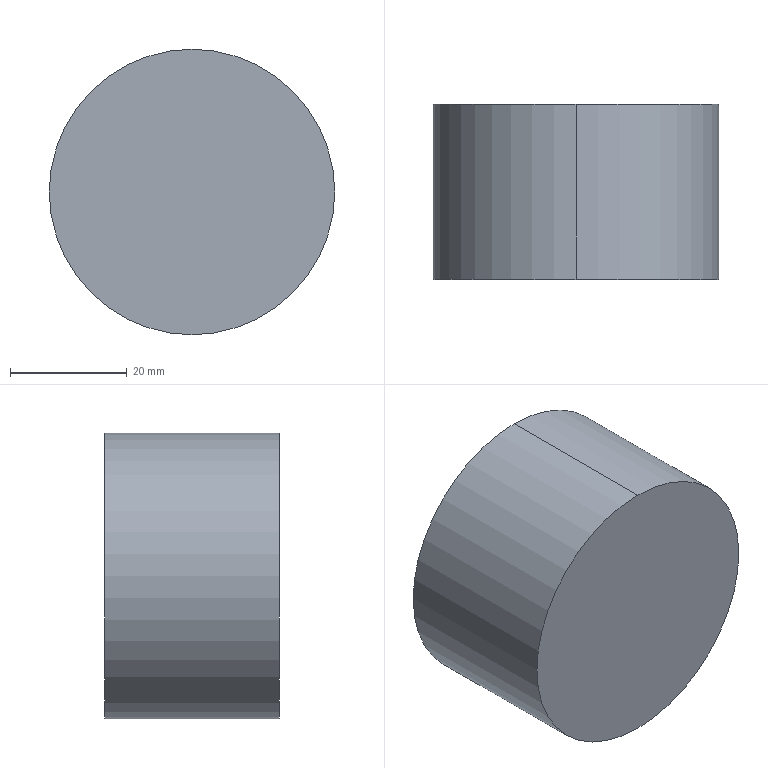Part | SolidWorks | features Extrusion 1 | 1 solid | 4 faces | box 48.94 x 30 x 48.94 mm | volume 56434 mm3 | cylinder 2 | plane 2 | commonest cylinder face diameters 48.94 x2
STEP:
#1=CARTESIAN_POINT('',(0.,30.,24.47));
#2=VERTEX_POINT('',#1);
#3=CARTESIAN_POINT('',(0.,30.,-24.47));
#4=VERTEX_POINT('',#3);
#5=CARTESIAN_POINT('',(0.,30.,0.));
#6=DIRECTION('',(0.,1.,0.));
#7=DIRECTION('',(0.,0.,1.));
#8=AXIS2_PLACEMENT_3D('',#5,#6,#7);
#9=CIRCLE('',#8,24.47);
#10=EDGE_CURVE('',#2,#4,#9,.T.);
#11=ORIENTED_EDGE('',*,*,#10,.F.);
#12=CARTESIAN_POINT('',(0.,0.,24.47));
#13=VERTEX_POINT('',#12);
#14=CARTESIAN_POINT('',(0.,30.,24.47));
#15=DIRECTION('',(0.,-1.,0.));
#16=VECTOR('',#15,1000.);
#17=LINE('',#14,#16);
#18=EDGE_CURVE('',#2,#13,#17,.T.);
#19=ORIENTED_EDGE('',*,*,#18,.T.);
#20=CARTESIAN_POINT('',(0.,0.,-24.47));
#21=VERTEX_POINT('',#20);
#22=CARTESIAN_POINT('',(0.,0.,0.));
#23=DIRECTION('',(0.,1.,0.));
#24=DIRECTION('',(0.,0.,1.));
#25=AXIS2_PLACEMENT_3D('',#22,#23,#24);
#26=CIRCLE('',#25,24.47);
#27=EDGE_CURVE('',#13,#21,#26,.T.);
#28=ORIENTED_EDGE('',*,*,#27,.T.);
#29=CARTESIAN_POINT('',(0.,30.,-24.47));
#30=DIRECTION('',(0.,-1.,0.));
#31=VECTOR('',#30,1000.);
#32=LINE('',#29,#31);
#33=EDGE_CURVE('',#4,#21,#32,.T.);
#34=ORIENTED_EDGE('',*,*,#33,.F.);
#35=EDGE_LOOP('',(#11,#19,#28,#34));
#36=FACE_OUTER_BOUND('',#35,.T.);
#37=CARTESIAN_POINT('',(0.,30.,0.));
#38=DIRECTION('',(0.,-1.,0.));
#39=DIRECTION('',(0.,0.,-1.));
#40=AXIS2_PLACEMENT_3D('',#37,#38,#39);
#41=CYLINDRICAL_SURFACE('',#40,24.47);
#42=ADVANCED_FACE('',(#36),#41,.T.);
#43=ORIENTED_EDGE('',*,*,#18,.F.);
#44=CARTESIAN_POINT('',(0.,30.,0.));
#45=DIRECTION('',(0.,1.,0.));
#46=DIRECTION('',(0.,0.,1.));
#47=AXIS2_PLACEMENT_3D('',#44,#45,#46);
#48=CIRCLE('',#47,24.47);
#49=EDGE_CURVE('',#4,#2,#48,.T.);
#50=ORIENTED_EDGE('',*,*,#49,.F.);
#51=ORIENTED_EDGE('',*,*,#33,.T.);
#52=CARTESIAN_POINT('',(0.,0.,0.));
#53=DIRECTION('',(0.,1.,0.));
#54=DIRECTION('',(0.,0.,1.));
#55=AXIS2_PLACEMENT_3D('',#52,#53,#54);
#56=CIRCLE('',#55,24.47);
#57=EDGE_CURVE('',#21,#13,#56,.T.);
#58=ORIENTED_EDGE('',*,*,#57,.T.);
#59=EDGE_LOOP('',(#43,#50,#51,#58));
#60=FACE_OUTER_BOUND('',#59,.T.);
#61=CARTESIAN_POINT('',(0.,30.,0.));
#62=DIRECTION('',(0.,-1.,0.));
#63=DIRECTION('',(0.,0.,-1.));
#64=AXIS2_PLACEMENT_3D('',#61,#62,#63);
#65=CYLINDRICAL_SURFACE('',#64,24.47);
#66=ADVANCED_FACE('',(#60),#65,.T.);
#67=ORIENTED_EDGE('',*,*,#49,.T.);
#68=ORIENTED_EDGE('',*,*,#10,.T.);
#69=EDGE_LOOP('',(#67,#68));
#70=FACE_OUTER_BOUND('',#69,.T.);
#71=CARTESIAN_POINT('',(0.,30.,0.));
#72=DIRECTION('',(0.,1.,0.));
#73=DIRECTION('',(0.,0.,1.));
#74=AXIS2_PLACEMENT_3D('',#71,#72,#73);
#75=PLANE('',#74);
#76=ADVANCED_FACE('',(#70),#75,.T.);
#77=ORIENTED_EDGE('',*,*,#57,.F.);
#78=ORIENTED_EDGE('',*,*,#27,.F.);
#79=EDGE_LOOP('',(#77,#78));
#80=FACE_OUTER_BOUND('',#79,.T.);
#81=CARTESIAN_POINT('',(0.,0.,0.));
#82=DIRECTION('',(0.,1.,0.));
#83=DIRECTION('',(0.,0.,1.));
#84=AXIS2_PLACEMENT_3D('',#81,#82,#83);
#85=PLANE('',#84);
#86=ADVANCED_FACE('',(#80),#85,.F.);
#87=CLOSED_SHELL('',(#42,#66,#76,#86));
#88=MANIFOLD_SOLID_BREP('',#87);
#89=CARTESIAN_POINT('',(0.,0.,0.));
#90=DIRECTION('',(0.,0.,1.));
#91=DIRECTION('',(1.,0.,0.));
#92=AXIS2_PLACEMENT_3D('',#89,#90,#91);
#93=(LENGTH_UNIT()NAMED_UNIT(*)SI_UNIT(.MILLI.,.METRE.));
#94=UNCERTAINTY_MEASURE_WITH_UNIT(LENGTH_MEASURE(0.00001),#93,'','');
#95=(NAMED_UNIT(*)PLANE_ANGLE_UNIT()SI_UNIT($,.RADIAN.));
#96=(NAMED_UNIT(*)SI_UNIT($,.STERADIAN.)SOLID_ANGLE_UNIT());
#97=(GEOMETRIC_REPRESENTATION_CONTEXT(3)GLOBAL_UNCERTAINTY_ASSIGNED_CONTEXT((#94))GLOBAL_UNIT_ASSIGNED_CONTEXT((#93,#95,#96))REPRESENTATION_CONTEXT('',''));
#98=ADVANCED_BREP_SHAPE_REPRESENTATION('',(#88,#92),#97);